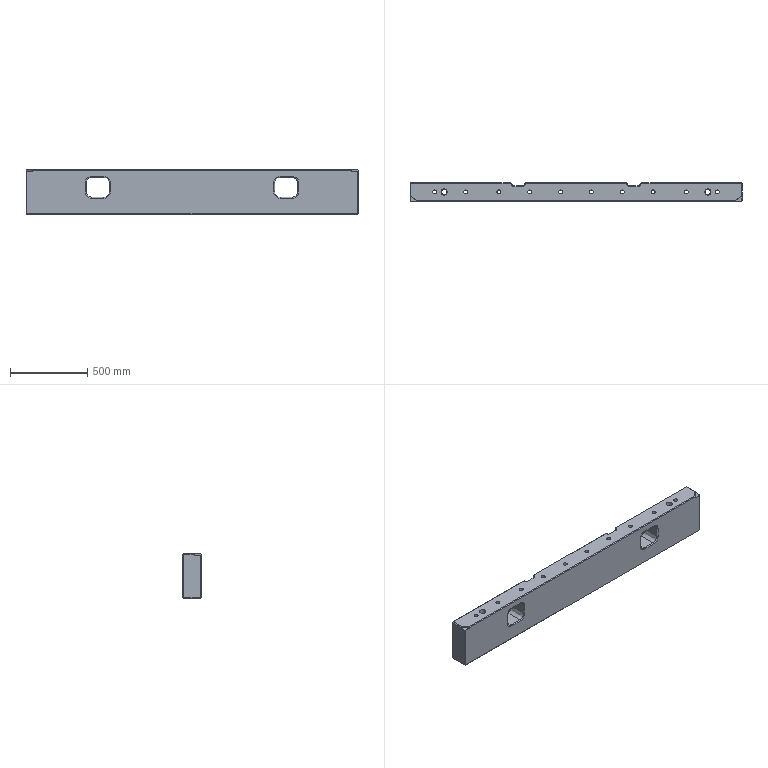Part | STEP file | solid 228 | 1 solid | 201 faces | box 2150 x 120 x 290 mm | volume 66813400 mm3 | plane 68 | cylinder 53 | cone 42 | spline 22 | torus 16 | commonest cylinder face diameters 26 x18 21 x11 39 x10 12 x8 40 x4 36 x2